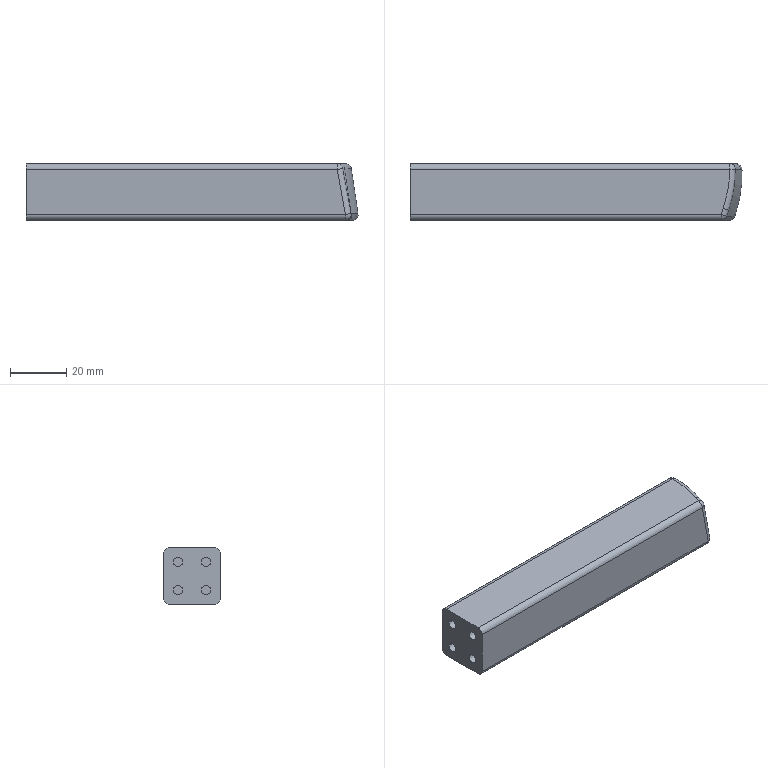Part | 1 solid | 36 faces | box 117.695 x 20 x 20.003 mm | volume 45374 mm3 | cylinder 14 | plane 9 | spline 8 | sphere 4 | torus 1 | commonest cylinder face diameters 3.3 x8 4 x5 5997 x1